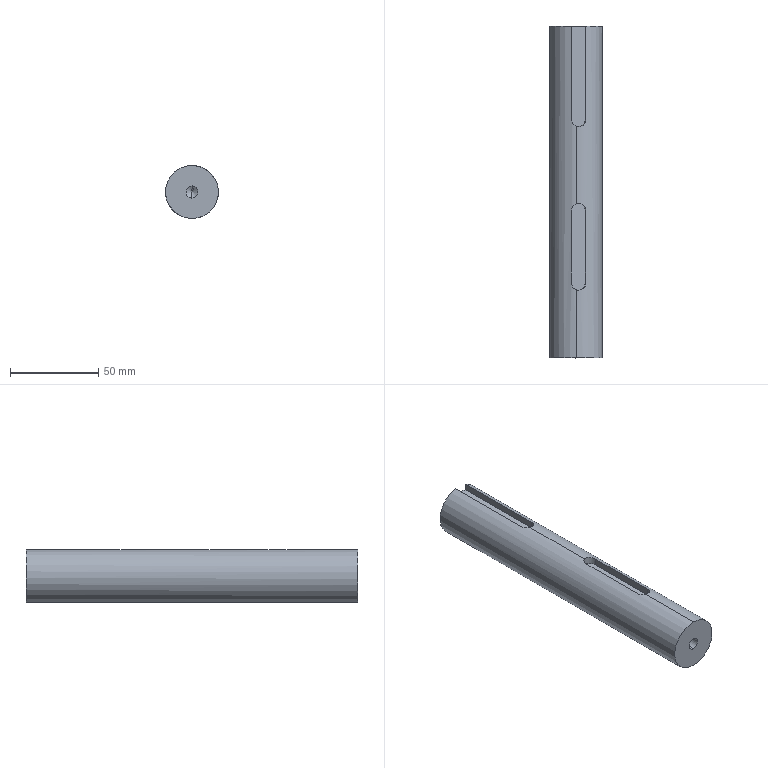Part | SolidWorks | features BaseBody 1 | 1 solid | 21 faces | box 30 x 188 x 30 mm | volume 126976 mm3 | cylinder 9 | plane 8 | cone 4 | commonest cylinder face diameters 6.8 x4 8 x3 30 x2
STEP:
#1=CARTESIAN_POINT('',(-1075.875,-37.235,-89.5));
#2=VERTEX_POINT('',#1);
#3=CARTESIAN_POINT('',(-1075.836,-39.278,-86.1));
#4=VERTEX_POINT('',#3);
#5=CARTESIAN_POINT('',(-1075.836,-39.278,-86.1));
#6=DIRECTION('',(0.009924,-0.515,0.8571));
#7=VECTOR('',#6,1000.);
#8=LINE('',#5,#7);
#9=EDGE_CURVE('',#2,#4,#8,.T.);
#10=ORIENTED_EDGE('',*,*,#9,.F.);
#11=CARTESIAN_POINT('',(-1075.915,-39.278,-92.9));
#12=VERTEX_POINT('',#11);
#13=CARTESIAN_POINT('',(-1075.915,-39.278,-92.9));
#14=DIRECTION('',(-0.009924,-0.515,-0.8571));
#15=VECTOR('',#14,1000.);
#16=LINE('',#13,#15);
#17=EDGE_CURVE('',#2,#12,#16,.T.);
#18=ORIENTED_EDGE('',*,*,#17,.T.);
#19=CARTESIAN_POINT('',(-1075.875,-39.278,-89.5));
#20=DIRECTION('',(0.,-1.,0.));
#21=DIRECTION('',(-0.01158,0.,-0.9999));
#22=AXIS2_PLACEMENT_3D('',#19,#20,#21);
#23=CIRCLE('',#22,3.4);
#24=EDGE_CURVE('',#12,#4,#23,.T.);
#25=ORIENTED_EDGE('',*,*,#24,.T.);
#26=EDGE_LOOP('',(#10,#18,#25));
#27=FACE_OUTER_BOUND('',#26,.T.);
#28=CARTESIAN_POINT('',(-1075.875,-39.278,-89.5));
#29=DIRECTION('',(0.,-1.,0.));
#30=DIRECTION('',(-0.01158,0.,-0.9999));
#31=AXIS2_PLACEMENT_3D('',#28,#29,#30);
#32=CONICAL_SURFACE('',#31,3.4,1.03);
#33=ADVANCED_FACE('',(#27),#32,.F.);
#34=CARTESIAN_POINT('',(-1075.875,77.18,-89.5));
#35=VERTEX_POINT('',#34);
#36=CARTESIAN_POINT('',(-1075.915,79.222,-92.9));
#37=VERTEX_POINT('',#36);
#38=CARTESIAN_POINT('',(-1075.915,79.222,-92.9));
#39=DIRECTION('',(-0.009924,0.515,-0.8571));
#40=VECTOR('',#39,1000.);
#41=LINE('',#38,#40);
#42=EDGE_CURVE('',#35,#37,#41,.T.);
#43=ORIENTED_EDGE('',*,*,#42,.F.);
#44=CARTESIAN_POINT('',(-1075.836,79.222,-86.1));
#45=VERTEX_POINT('',#44);
#46=CARTESIAN_POINT('',(-1075.836,79.222,-86.1));
#47=DIRECTION('',(0.009924,0.515,0.8571));
#48=VECTOR('',#47,1000.);
#49=LINE('',#46,#48);
#50=EDGE_CURVE('',#35,#45,#49,.T.);
#51=ORIENTED_EDGE('',*,*,#50,.T.);
#52=CARTESIAN_POINT('',(-1075.875,79.222,-89.5));
#53=DIRECTION('',(0.,1.,0.));
#54=DIRECTION('',(0.01158,0.,0.9999));
#55=AXIS2_PLACEMENT_3D('',#52,#53,#54);
#56=CIRCLE('',#55,3.4);
#57=EDGE_CURVE('',#45,#37,#56,.T.);
#58=ORIENTED_EDGE('',*,*,#57,.T.);
#59=EDGE_LOOP('',(#43,#51,#58));
#60=FACE_OUTER_BOUND('',#59,.T.);
#61=CARTESIAN_POINT('',(-1075.875,79.222,-89.5));
#62=DIRECTION('',(0.,1.,0.));
#63=DIRECTION('',(0.01158,0.,0.9999));
#64=AXIS2_PLACEMENT_3D('',#61,#62,#63);
#65=CONICAL_SURFACE('',#64,3.4,1.03);
#66=ADVANCED_FACE('',(#60),#65,.F.);
#67=CARTESIAN_POINT('',(-1075.836,-59.028,-86.1));
#68=VERTEX_POINT('',#67);
#69=CARTESIAN_POINT('',(-1075.836,-59.028,-86.1));
#70=DIRECTION('',(0.,-1.,0.));
#71=VECTOR('',#70,1000.);
#72=LINE('',#69,#71);
#73=EDGE_CURVE('',#4,#68,#72,.T.);
#74=ORIENTED_EDGE('',*,*,#73,.F.);
#75=ORIENTED_EDGE('',*,*,#24,.F.);
#76=CARTESIAN_POINT('',(-1075.915,-59.028,-92.9));
#77=VERTEX_POINT('',#76);
#78=CARTESIAN_POINT('',(-1075.915,-59.028,-92.9));
#79=DIRECTION('',(0.,-1.,0.));
#80=VECTOR('',#79,1000.);
#81=LINE('',#78,#80);
#82=EDGE_CURVE('',#12,#77,#81,.T.);
#83=ORIENTED_EDGE('',*,*,#82,.T.);
#84=CARTESIAN_POINT('',(-1075.875,-59.028,-89.5));
#85=DIRECTION('',(0.,-1.,0.));
#86=DIRECTION('',(-0.01158,0.,-0.9999));
#87=AXIS2_PLACEMENT_3D('',#84,#85,#86);
#88=CIRCLE('',#87,3.4);
#89=EDGE_CURVE('',#77,#68,#88,.T.);
#90=ORIENTED_EDGE('',*,*,#89,.T.);
#91=EDGE_LOOP('',(#74,#75,#83,#90));
#92=FACE_OUTER_BOUND('',#91,.T.);
#93=CARTESIAN_POINT('',(-1075.875,-59.028,-89.5));
#94=DIRECTION('',(0.,-1.,0.));
#95=DIRECTION('',(-0.01158,0.,-0.9999));
#96=AXIS2_PLACEMENT_3D('',#93,#94,#95);
#97=CYLINDRICAL_SURFACE('',#96,3.4);
#98=ADVANCED_FACE('',(#92),#97,.F.);
#99=CARTESIAN_POINT('',(-1078.679,-16.675,-78.33));
#100=VERTEX_POINT('',#99);
#101=CARTESIAN_POINT('',(-1070.726,-16.675,-79.198));
#102=VERTEX_POINT('',#101);
#103=CARTESIAN_POINT('',(-1074.703,-16.675,-78.764));
#104=DIRECTION('',(0.1086,0.,0.9941));
#105=DIRECTION('',(-0.9941,0.,0.1086));
#106=AXIS2_PLACEMENT_3D('',#103,#104,#105);
#107=CIRCLE('',#106,4.);
#108=EDGE_CURVE('',#100,#102,#107,.T.);
#109=ORIENTED_EDGE('',*,*,#108,.T.);
#110=CARTESIAN_POINT('',(-1070.726,24.625,-79.198));
#111=VERTEX_POINT('',#110);
#112=CARTESIAN_POINT('',(-1070.726,-16.675,-79.198));
#113=DIRECTION('',(0.,1.,0.));
#114=VECTOR('',#113,1000.);
#115=LINE('',#112,#114);
#116=EDGE_CURVE('',#102,#111,#115,.T.);
#117=ORIENTED_EDGE('',*,*,#116,.T.);
#118=CARTESIAN_POINT('',(-1078.679,24.625,-78.33));
#119=VERTEX_POINT('',#118);
#120=CARTESIAN_POINT('',(-1074.703,24.625,-78.764));
#121=DIRECTION('',(0.1086,0.,0.9941));
#122=DIRECTION('',(-0.9941,0.,0.1086));
#123=AXIS2_PLACEMENT_3D('',#120,#121,#122);
#124=CIRCLE('',#123,4.);
#125=EDGE_CURVE('',#111,#119,#124,.T.);
#126=ORIENTED_EDGE('',*,*,#125,.T.);
#127=CARTESIAN_POINT('',(-1078.679,24.625,-78.33));
#128=DIRECTION('',(0.,-1.,0.));
#129=VECTOR('',#128,1000.);
#130=LINE('',#127,#129);
#131=EDGE_CURVE('',#119,#100,#130,.T.);
#132=ORIENTED_EDGE('',*,*,#131,.T.);
#133=EDGE_LOOP('',(#109,#117,#126,#132));
#134=FACE_OUTER_BOUND('',#133,.T.);
#135=CARTESIAN_POINT('',(-1074.703,24.625,-78.764));
#136=DIRECTION('',(0.1086,0.,0.9941));
#137=DIRECTION('',(0.,1.,0.));
#138=AXIS2_PLACEMENT_3D('',#135,#136,#137);
#139=PLANE('',#138);
#140=ADVANCED_FACE('',(#134),#139,.T.);
#141=CARTESIAN_POINT('',(-1070.329,24.625,-75.563));
#142=VERTEX_POINT('',#141);
#143=CARTESIAN_POINT('',(-1070.726,24.625,-79.198));
#144=DIRECTION('',(-0.1086,0.,-0.9941));
#145=VECTOR('',#144,1000.);
#146=LINE('',#143,#145);
#147=EDGE_CURVE('',#142,#111,#146,.T.);
#148=ORIENTED_EDGE('',*,*,#147,.T.);
#149=ORIENTED_EDGE('',*,*,#116,.F.);
#150=CARTESIAN_POINT('',(-1070.329,-16.675,-75.563));
#151=VERTEX_POINT('',#150);
#152=CARTESIAN_POINT('',(-1070.726,-16.675,-79.198));
#153=DIRECTION('',(0.1086,0.,0.9941));
#154=VECTOR('',#153,1000.);
#155=LINE('',#152,#154);
#156=EDGE_CURVE('',#102,#151,#155,.T.);
#157=ORIENTED_EDGE('',*,*,#156,.T.);
#158=CARTESIAN_POINT('',(-1070.329,-91.028,-75.563));
#159=DIRECTION('',(0.,-1.,0.));
#160=VECTOR('',#159,1000.);
#161=LINE('',#158,#160);
#162=EDGE_CURVE('',#142,#151,#161,.T.);
#163=ORIENTED_EDGE('',*,*,#162,.F.);
#164=EDGE_LOOP('',(#148,#149,#157,#163));
#165=FACE_OUTER_BOUND('',#164,.T.);
#166=CARTESIAN_POINT('',(-1070.726,-16.675,-79.198));
#167=DIRECTION('',(0.9941,0.,-0.1086));
#168=DIRECTION('',(0.,1.,0.));
#169=AXIS2_PLACEMENT_3D('',#166,#167,#168);
#170=PLANE('',#169);
#171=ADVANCED_FACE('',(#165),#170,.F.);
#172=CARTESIAN_POINT('',(-1075.915,128.972,-92.9));
#173=VERTEX_POINT('',#172);
#174=CARTESIAN_POINT('',(-1075.915,98.972,-92.9));
#175=DIRECTION('',(0.,1.,0.));
#176=VECTOR('',#175,1000.);
#177=LINE('',#174,#176);
#178=EDGE_CURVE('',#37,#173,#177,.T.);
#179=ORIENTED_EDGE('',*,*,#178,.F.);
#180=ORIENTED_EDGE('',*,*,#57,.F.);
#181=CARTESIAN_POINT('',(-1075.836,128.972,-86.1));
#182=VERTEX_POINT('',#181);
#183=CARTESIAN_POINT('',(-1075.836,98.972,-86.1));
#184=DIRECTION('',(0.,1.,0.));
#185=VECTOR('',#184,1000.);
#186=LINE('',#183,#185);
#187=EDGE_CURVE('',#45,#182,#186,.T.);
#188=ORIENTED_EDGE('',*,*,#187,.T.);
#189=CARTESIAN_POINT('',(-1075.875,128.972,-89.5));
#190=DIRECTION('',(0.,-1.,0.));
#191=DIRECTION('',(0.01158,0.,0.9999));
#192=AXIS2_PLACEMENT_3D('',#189,#190,#191);
#193=CIRCLE('',#192,3.4);
#194=EDGE_CURVE('',#173,#182,#193,.T.);
#195=ORIENTED_EDGE('',*,*,#194,.F.);
#196=EDGE_LOOP('',(#179,#180,#188,#195));
#197=FACE_OUTER_BOUND('',#196,.T.);
#198=CARTESIAN_POINT('',(-1075.875,98.972,-89.5));
#199=DIRECTION('',(0.,1.,0.));
#200=DIRECTION('',(0.01158,0.,0.9999));
#201=AXIS2_PLACEMENT_3D('',#198,#199,#200);
#202=CYLINDRICAL_SURFACE('',#201,3.4);
#203=ADVANCED_FACE('',(#197),#202,.F.);
#204=CARTESIAN_POINT('',(-1070.726,128.972,-79.198));
#205=VERTEX_POINT('',#204);
#206=CARTESIAN_POINT('',(-1070.329,128.972,-75.563));
#207=VERTEX_POINT('',#206);
#208=CARTESIAN_POINT('',(-1070.726,128.972,-79.198));
#209=DIRECTION('',(0.1086,0.,0.9941));
#210=VECTOR('',#209,1000.);
#211=LINE('',#208,#210);
#212=EDGE_CURVE('',#205,#207,#211,.T.);
#213=ORIENTED_EDGE('',*,*,#212,.F.);
#214=CARTESIAN_POINT('',(-1070.726,75.972,-79.198));
#215=VERTEX_POINT('',#214);
#216=CARTESIAN_POINT('',(-1070.726,75.972,-79.198));
#217=DIRECTION('',(0.,1.,0.));
#218=VECTOR('',#217,1000.);
#219=LINE('',#216,#218);
#220=EDGE_CURVE('',#215,#205,#219,.T.);
#221=ORIENTED_EDGE('',*,*,#220,.F.);
#222=CARTESIAN_POINT('',(-1070.329,75.972,-75.563));
#223=VERTEX_POINT('',#222);
#224=CARTESIAN_POINT('',(-1070.726,75.972,-79.198));
#225=DIRECTION('',(0.1086,0.,0.9941));
#226=VECTOR('',#225,1000.);
#227=LINE('',#224,#226);
#228=EDGE_CURVE('',#215,#223,#227,.T.);
#229=ORIENTED_EDGE('',*,*,#228,.T.);
#230=CARTESIAN_POINT('',(-1070.329,-91.028,-75.563));
#231=DIRECTION('',(0.,-1.,0.));
#232=VECTOR('',#231,1000.);
#233=LINE('',#230,#232);
#234=EDGE_CURVE('',#207,#223,#233,.T.);
#235=ORIENTED_EDGE('',*,*,#234,.F.);
#236=EDGE_LOOP('',(#213,#221,#229,#235));
#237=FACE_OUTER_BOUND('',#236,.T.);
#238=CARTESIAN_POINT('',(-1070.726,75.972,-79.198));
#239=DIRECTION('',(0.9941,0.,-0.1086));
#240=DIRECTION('',(0.,1.,0.));
#241=AXIS2_PLACEMENT_3D('',#238,#239,#240);
#242=PLANE('',#241);
#243=ADVANCED_FACE('',(#237),#242,.F.);
#244=CARTESIAN_POINT('',(-1078.679,75.972,-78.33));
#245=VERTEX_POINT('',#244);
#246=CARTESIAN_POINT('',(-1074.703,75.972,-78.764));
#247=DIRECTION('',(0.1086,0.,0.9941));
#248=DIRECTION('',(-0.9941,0.,0.1086));
#249=AXIS2_PLACEMENT_3D('',#246,#247,#248);
#250=CIRCLE('',#249,4.);
#251=EDGE_CURVE('',#245,#215,#250,.T.);
#252=ORIENTED_EDGE('',*,*,#251,.T.);
#253=ORIENTED_EDGE('',*,*,#220,.T.);
#254=CARTESIAN_POINT('',(-1078.679,128.972,-78.33));
#255=VERTEX_POINT('',#254);
#256=CARTESIAN_POINT('',(-1074.703,128.972,-78.764));
#257=DIRECTION('',(0.9941,0.,-0.1086));
#258=VECTOR('',#257,1000.);
#259=LINE('',#256,#258);
#260=EDGE_CURVE('',#255,#205,#259,.T.);
#261=ORIENTED_EDGE('',*,*,#260,.F.);
#262=CARTESIAN_POINT('',(-1078.679,98.972,-78.33));
#263=DIRECTION('',(0.,-1.,0.));
#264=VECTOR('',#263,1000.);
#265=LINE('',#262,#264);
#266=EDGE_CURVE('',#255,#245,#265,.T.);
#267=ORIENTED_EDGE('',*,*,#266,.T.);
#268=EDGE_LOOP('',(#252,#253,#261,#267));
#269=FACE_OUTER_BOUND('',#268,.T.);
#270=CARTESIAN_POINT('',(-1074.703,75.972,-78.764));
#271=DIRECTION('',(0.1086,0.,0.9941));
#272=DIRECTION('',(0.,1.,0.));
#273=AXIS2_PLACEMENT_3D('',#270,#271,#272);
#274=PLANE('',#273);
#275=ADVANCED_FACE('',(#269),#274,.T.);
#276=CARTESIAN_POINT('',(-1075.702,-59.028,-74.501));
#277=VERTEX_POINT('',#276);
#278=CARTESIAN_POINT('',(-1076.049,-59.028,-104.499));
#279=VERTEX_POINT('',#278);
#280=CARTESIAN_POINT('',(-1075.875,-59.028,-89.5));
#281=DIRECTION('',(0.,1.,0.));
#282=DIRECTION('',(0.01158,0.,0.9999));
#283=AXIS2_PLACEMENT_3D('',#280,#281,#282);
#284=CIRCLE('',#283,15.);
#285=EDGE_CURVE('',#277,#279,#284,.T.);
#286=ORIENTED_EDGE('',*,*,#285,.F.);
#287=CARTESIAN_POINT('',(-1075.875,-59.028,-89.5));
#288=DIRECTION('',(0.,1.,0.));
#289=DIRECTION('',(0.01158,0.,0.9999));
#290=AXIS2_PLACEMENT_3D('',#287,#288,#289);
#291=CIRCLE('',#290,15.);
#292=EDGE_CURVE('',#279,#277,#291,.T.);
#293=ORIENTED_EDGE('',*,*,#292,.F.);
#294=EDGE_LOOP('',(#286,#293));
#295=FACE_OUTER_BOUND('',#294,.T.);
#296=ORIENTED_EDGE('',*,*,#89,.F.);
#297=CARTESIAN_POINT('',(-1075.875,-59.028,-89.5));
#298=DIRECTION('',(0.,-1.,0.));
#299=DIRECTION('',(-0.01158,0.,-0.9999));
#300=AXIS2_PLACEMENT_3D('',#297,#298,#299);
#301=CIRCLE('',#300,3.4);
#302=EDGE_CURVE('',#68,#77,#301,.T.);
#303=ORIENTED_EDGE('',*,*,#302,.F.);
#304=EDGE_LOOP('',(#296,#303));
#305=FACE_BOUND('',#304,.T.);
#306=CARTESIAN_POINT('',(-1075.875,-59.028,-89.5));
#307=DIRECTION('',(0.,1.,0.));
#308=DIRECTION('',(0.01158,0.,0.9999));
#309=AXIS2_PLACEMENT_3D('',#306,#307,#308);
#310=PLANE('',#309);
#311=ADVANCED_FACE('',(#295,#305),#310,.F.);
#312=ORIENTED_EDGE('',*,*,#156,.F.);
#313=ORIENTED_EDGE('',*,*,#108,.F.);
#314=CARTESIAN_POINT('',(-1078.282,-16.675,-74.694));
#315=VERTEX_POINT('',#314);
#316=CARTESIAN_POINT('',(-1078.679,-16.675,-78.33));
#317=DIRECTION('',(0.1086,0.,0.9941));
#318=VECTOR('',#317,1000.);
#319=LINE('',#316,#318);
#320=EDGE_CURVE('',#100,#315,#319,.T.);
#321=ORIENTED_EDGE('',*,*,#320,.T.);
#322=CARTESIAN_POINT('',(-1075.702,-20.401,-74.501));
#323=VERTEX_POINT('',#322);
#324=CARTESIAN_POINT('',(-1075.702,-20.401,-74.501));
#325=CARTESIAN_POINT('',(-1076.077,-20.255,-74.497));
#326=CARTESIAN_POINT('',(-1076.424,-20.057,-74.507));
#327=CARTESIAN_POINT('',(-1076.901,-19.683,-74.534));
#328=CARTESIAN_POINT('',(-1077.049,-19.548,-74.545));
#329=CARTESIAN_POINT('',(-1077.324,-19.258,-74.569));
#330=CARTESIAN_POINT('',(-1077.449,-19.104,-74.582));
#331=CARTESIAN_POINT('',(-1077.681,-18.772,-74.609));
#332=CARTESIAN_POINT('',(-1077.784,-18.599,-74.622));
#333=CARTESIAN_POINT('',(-1077.917,-18.331,-74.639));
#334=CARTESIAN_POINT('',(-1077.957,-18.24,-74.645));
#335=CARTESIAN_POINT('',(-1078.032,-18.055,-74.656));
#336=CARTESIAN_POINT('',(-1078.066,-17.962,-74.661));
#337=CARTESIAN_POINT('',(-1078.22,-17.477,-74.684));
#338=CARTESIAN_POINT('',(-1078.282,-17.08,-74.694));
#339=CARTESIAN_POINT('',(-1078.282,-16.675,-74.694));
#340=B_SPLINE_CURVE_WITH_KNOTS('',3,(#324,#325,#326,#327,#328,#329,#330,#331,#332,#333,#334,#335,#336,#337,#338,#339),.UNSPECIFIED.,.F.,.F.,(4,2,2,2,2,2,2,4),(0.,0.25,0.375,0.5,0.625,0.6875,0.75,1.),.UNSPECIFIED.);
#341=EDGE_CURVE('',#323,#315,#340,.T.);
#342=ORIENTED_EDGE('',*,*,#341,.F.);
#343=CARTESIAN_POINT('',(-1070.329,-16.675,-75.563));
#344=CARTESIAN_POINT('',(-1070.329,-17.001,-75.563));
#345=CARTESIAN_POINT('',(-1070.367,-17.323,-75.548));
#346=CARTESIAN_POINT('',(-1070.481,-17.797,-75.504));
#347=CARTESIAN_POINT('',(-1070.527,-17.951,-75.486));
#348=CARTESIAN_POINT('',(-1070.639,-18.253,-75.444));
#349=CARTESIAN_POINT('',(-1070.704,-18.402,-75.419));
#350=CARTESIAN_POINT('',(-1070.851,-18.688,-75.366));
#351=CARTESIAN_POINT('',(-1070.932,-18.826,-75.338));
#352=CARTESIAN_POINT('',(-1071.11,-19.09,-75.277));
#353=CARTESIAN_POINT('',(-1071.208,-19.218,-75.244));
#354=CARTESIAN_POINT('',(-1071.521,-19.579,-75.144));
#355=CARTESIAN_POINT('',(-1071.755,-19.791,-75.074));
#356=CARTESIAN_POINT('',(-1072.279,-20.158,-74.935));
#357=CARTESIAN_POINT('',(-1072.557,-20.306,-74.868));
#358=CARTESIAN_POINT('',(-1073.158,-20.535,-74.745));
#359=CARTESIAN_POINT('',(-1073.469,-20.611,-74.691));
#360=CARTESIAN_POINT('',(-1074.112,-20.686,-74.6));
#361=CARTESIAN_POINT('',(-1074.434,-20.684,-74.566));
#362=CARTESIAN_POINT('',(-1075.081,-20.6,-74.518));
#363=CARTESIAN_POINT('',(-1075.396,-20.52,-74.505));
#364=CARTESIAN_POINT('',(-1075.702,-20.401,-74.501));
#365=B_SPLINE_CURVE_WITH_KNOTS('',3,(#343,#344,#345,#346,#347,#348,#349,#350,#351,#352,#353,#354,#355,#356,#357,#358,#359,#360,#361,#362,#363,#364),.UNSPECIFIED.,.F.,.F.,(4,2,2,2,2,2,2,2,2,2,4),(0.,0.125,0.1875,0.25,0.3125,0.375,0.5,0.625,0.75,0.875,1.),.UNSPECIFIED.);
#366=EDGE_CURVE('',#151,#323,#365,.T.);
#367=ORIENTED_EDGE('',*,*,#366,.F.);
#368=EDGE_LOOP('',(#312,#313,#321,#342,#367));
#369=FACE_OUTER_BOUND('',#368,.T.);
#370=CARTESIAN_POINT('',(-1074.703,-16.675,-78.764));
#371=DIRECTION('',(0.1086,0.,0.9941));
#372=DIRECTION('',(-0.9941,0.,0.1086));
#373=AXIS2_PLACEMENT_3D('',#370,#371,#372);
#374=CYLINDRICAL_SURFACE('',#373,4.);
#375=ADVANCED_FACE('',(#369),#374,.F.);
#376=ORIENTED_EDGE('',*,*,#320,.F.);
#377=ORIENTED_EDGE('',*,*,#131,.F.);
#378=CARTESIAN_POINT('',(-1078.282,24.625,-74.694));
#379=VERTEX_POINT('',#378);
#380=CARTESIAN_POINT('',(-1078.679,24.625,-78.33));
#381=DIRECTION('',(0.1086,0.,0.9941));
#382=VECTOR('',#381,1000.);
#383=LINE('',#380,#382);
#384=EDGE_CURVE('',#119,#379,#383,.T.);
#385=ORIENTED_EDGE('',*,*,#384,.T.);
#386=CARTESIAN_POINT('',(-1078.282,-91.028,-74.694));
#387=DIRECTION('',(0.,1.,0.));
#388=VECTOR('',#387,1000.);
#389=LINE('',#386,#388);
#390=EDGE_CURVE('',#315,#379,#389,.T.);
#391=ORIENTED_EDGE('',*,*,#390,.F.);
#392=EDGE_LOOP('',(#376,#377,#385,#391));
#393=FACE_OUTER_BOUND('',#392,.T.);
#394=CARTESIAN_POINT('',(-1078.679,24.625,-78.33));
#395=DIRECTION('',(-0.9941,0.,0.1086));
#396=DIRECTION('',(-0.1086,0.,-0.9941));
#397=AXIS2_PLACEMENT_3D('',#394,#395,#396);
#398=PLANE('',#397);
#399=ADVANCED_FACE('',(#393),#398,.F.);
#400=ORIENTED_EDGE('',*,*,#384,.F.);
#401=ORIENTED_EDGE('',*,*,#125,.F.);
#402=ORIENTED_EDGE('',*,*,#147,.F.);
#403=CARTESIAN_POINT('',(-1075.702,28.351,-74.501));
#404=VERTEX_POINT('',#403);
#405=CARTESIAN_POINT('',(-1075.702,28.351,-74.501));
#406=CARTESIAN_POINT('',(-1075.397,28.469,-74.505));
#407=CARTESIAN_POINT('',(-1075.085,28.549,-74.517));
#408=CARTESIAN_POINT('',(-1074.438,28.634,-74.566));
#409=CARTESIAN_POINT('',(-1074.114,28.636,-74.6));
#410=CARTESIAN_POINT('',(-1073.632,28.58,-74.668));
#411=CARTESIAN_POINT('',(-1073.474,28.552,-74.693));
#412=CARTESIAN_POINT('',(-1073.163,28.476,-74.746));
#413=CARTESIAN_POINT('',(-1073.009,28.428,-74.776));
#414=CARTESIAN_POINT('',(-1072.561,28.257,-74.868));
#415=CARTESIAN_POINT('',(-1072.28,28.109,-74.935));
#416=CARTESIAN_POINT('',(-1071.758,27.743,-75.074));
#417=CARTESIAN_POINT('',(-1071.524,27.532,-75.143));
#418=CARTESIAN_POINT('',(-1071.208,27.168,-75.244));
#419=CARTESIAN_POINT('',(-1071.111,27.041,-75.276));
#420=CARTESIAN_POINT('',(-1070.933,26.777,-75.337));
#421=CARTESIAN_POINT('',(-1070.852,26.64,-75.366));
#422=CARTESIAN_POINT('',(-1070.704,26.352,-75.419));
#423=CARTESIAN_POINT('',(-1070.639,26.204,-75.443));
#424=CARTESIAN_POINT('',(-1070.528,25.903,-75.485));
#425=CARTESIAN_POINT('',(-1070.482,25.75,-75.503));
#426=CARTESIAN_POINT('',(-1070.367,25.274,-75.548));
#427=CARTESIAN_POINT('',(-1070.329,24.951,-75.563));
#428=CARTESIAN_POINT('',(-1070.329,24.625,-75.563));
#429=B_SPLINE_CURVE_WITH_KNOTS('',3,(#405,#406,#407,#408,#409,#410,#411,#412,#413,#414,#415,#416,#417,#418,#419,#420,#421,#422,#423,#424,#425,#426,#427,#428),.UNSPECIFIED.,.F.,.F.,(4,2,2,2,2,2,2,2,2,2,2,4),(0.,0.125,0.25,0.3125,0.375,0.5,0.625,0.6875,0.75,0.8125,0.875,1.),.UNSPECIFIED.);
#430=EDGE_CURVE('',#404,#142,#429,.T.);
#431=ORIENTED_EDGE('',*,*,#430,.F.);
#432=CARTESIAN_POINT('',(-1078.282,24.625,-74.694));
#433=CARTESIAN_POINT('',(-1078.282,24.826,-74.694));
#434=CARTESIAN_POINT('',(-1078.267,25.026,-74.692));
#435=CARTESIAN_POINT('',(-1078.206,25.42,-74.682));
#436=CARTESIAN_POINT('',(-1078.159,25.617,-74.675));
#437=CARTESIAN_POINT('',(-1078.038,26.,-74.657));
#438=CARTESIAN_POINT('',(-1077.964,26.185,-74.646));
#439=CARTESIAN_POINT('',(-1077.787,26.543,-74.622));
#440=CARTESIAN_POINT('',(-1077.684,26.717,-74.609));
#441=CARTESIAN_POINT('',(-1077.339,27.212,-74.57));
#442=CARTESIAN_POINT('',(-1077.067,27.501,-74.544));
#443=CARTESIAN_POINT('',(-1076.428,28.004,-74.507));
#444=CARTESIAN_POINT('',(-1076.079,28.204,-74.497));
#445=CARTESIAN_POINT('',(-1075.702,28.351,-74.501));
#446=B_SPLINE_CURVE_WITH_KNOTS('',3,(#432,#433,#434,#435,#436,#437,#438,#439,#440,#441,#442,#443,#444,#445),.UNSPECIFIED.,.F.,.F.,(4,2,2,2,2,2,4),(0.,0.125,0.25,0.375,0.5,0.75,1.),.UNSPECIFIED.);
#447=EDGE_CURVE('',#379,#404,#446,.T.);
#448=ORIENTED_EDGE('',*,*,#447,.F.);
#449=EDGE_LOOP('',(#400,#401,#402,#431,#448));
#450=FACE_OUTER_BOUND('',#449,.T.);
#451=CARTESIAN_POINT('',(-1074.703,24.625,-78.764));
#452=DIRECTION('',(0.1086,0.,0.9941));
#453=DIRECTION('',(-0.9941,0.,0.1086));
#454=AXIS2_PLACEMENT_3D('',#451,#452,#453);
#455=CYLINDRICAL_SURFACE('',#454,4.);
#456=ADVANCED_FACE('',(#450),#455,.F.);
#457=ORIENTED_EDGE('',*,*,#228,.F.);
#458=ORIENTED_EDGE('',*,*,#251,.F.);
#459=CARTESIAN_POINT('',(-1078.282,75.972,-74.694));
#460=VERTEX_POINT('',#459);
#461=CARTESIAN_POINT('',(-1078.679,75.972,-78.33));
#462=DIRECTION('',(0.1086,0.,0.9941));
#463=VECTOR('',#462,1000.);
#464=LINE('',#461,#463);
#465=EDGE_CURVE('',#245,#460,#464,.T.);
#466=ORIENTED_EDGE('',*,*,#465,.T.);
#467=CARTESIAN_POINT('',(-1075.702,72.247,-74.501));
#468=VERTEX_POINT('',#467);
#469=CARTESIAN_POINT('',(-1075.702,72.247,-74.501));
#470=CARTESIAN_POINT('',(-1076.077,72.393,-74.497));
#471=CARTESIAN_POINT('',(-1076.424,72.59,-74.507));
#472=CARTESIAN_POINT('',(-1076.901,72.965,-74.534));
#473=CARTESIAN_POINT('',(-1077.049,73.1,-74.545));
#474=CARTESIAN_POINT('',(-1077.324,73.39,-74.569));
#475=CARTESIAN_POINT('',(-1077.449,73.543,-74.582));
#476=CARTESIAN_POINT('',(-1077.681,73.876,-74.609));
#477=CARTESIAN_POINT('',(-1077.784,74.048,-74.622));
#478=CARTESIAN_POINT('',(-1077.917,74.317,-74.639));
#479=CARTESIAN_POINT('',(-1077.957,74.408,-74.645));
#480=CARTESIAN_POINT('',(-1078.032,74.593,-74.656));
#481=CARTESIAN_POINT('',(-1078.066,74.685,-74.661));
#482=CARTESIAN_POINT('',(-1078.22,75.171,-74.684));
#483=CARTESIAN_POINT('',(-1078.282,75.567,-74.694));
#484=CARTESIAN_POINT('',(-1078.282,75.972,-74.694));
#485=B_SPLINE_CURVE_WITH_KNOTS('',3,(#469,#470,#471,#472,#473,#474,#475,#476,#477,#478,#479,#480,#481,#482,#483,#484),.UNSPECIFIED.,.F.,.F.,(4,2,2,2,2,2,2,4),(0.,0.25,0.375,0.5,0.625,0.6875,0.75,1.),.UNSPECIFIED.);
#486=EDGE_CURVE('',#468,#460,#485,.T.);
#487=ORIENTED_EDGE('',*,*,#486,.F.);
#488=CARTESIAN_POINT('',(-1070.329,75.972,-75.563));
#489=CARTESIAN_POINT('',(-1070.329,75.647,-75.563));
#490=CARTESIAN_POINT('',(-1070.367,75.324,-75.548));
#491=CARTESIAN_POINT('',(-1070.481,74.851,-75.504));
#492=CARTESIAN_POINT('',(-1070.527,74.697,-75.486));
#493=CARTESIAN_POINT('',(-1070.639,74.395,-75.444));
#494=CARTESIAN_POINT('',(-1070.704,74.245,-75.419));
#495=CARTESIAN_POINT('',(-1070.851,73.959,-75.366));
#496=CARTESIAN_POINT('',(-1070.932,73.822,-75.338));
#497=CARTESIAN_POINT('',(-1071.11,73.557,-75.277));
#498=CARTESIAN_POINT('',(-1071.208,73.429,-75.244));
#499=CARTESIAN_POINT('',(-1071.521,73.068,-75.144));
#500=CARTESIAN_POINT('',(-1071.755,72.857,-75.074));
#501=CARTESIAN_POINT('',(-1072.279,72.49,-74.935));
#502=CARTESIAN_POINT('',(-1072.557,72.342,-74.868));
#503=CARTESIAN_POINT('',(-1073.158,72.112,-74.745));
#504=CARTESIAN_POINT('',(-1073.469,72.036,-74.691));
#505=CARTESIAN_POINT('',(-1074.112,71.961,-74.6));
#506=CARTESIAN_POINT('',(-1074.434,71.964,-74.566));
#507=CARTESIAN_POINT('',(-1075.081,72.047,-74.518));
#508=CARTESIAN_POINT('',(-1075.396,72.128,-74.505));
#509=CARTESIAN_POINT('',(-1075.702,72.247,-74.501));
#510=B_SPLINE_CURVE_WITH_KNOTS('',3,(#488,#489,#490,#491,#492,#493,#494,#495,#496,#497,#498,#499,#500,#501,#502,#503,#504,#505,#506,#507,#508,#509),.UNSPECIFIED.,.F.,.F.,(4,2,2,2,2,2,2,2,2,2,4),(0.,0.125,0.1875,0.25,0.3125,0.375,0.5,0.625,0.75,0.875,1.),.UNSPECIFIED.);
#511=EDGE_CURVE('',#223,#468,#510,.T.);
#512=ORIENTED_EDGE('',*,*,#511,.F.);
#513=EDGE_LOOP('',(#457,#458,#466,#487,#512));
#514=FACE_OUTER_BOUND('',#513,.T.);
#515=CARTESIAN_POINT('',(-1074.703,75.972,-78.764));
#516=DIRECTION('',(0.1086,0.,0.9941));
#517=DIRECTION('',(-0.9941,0.,0.1086));
#518=AXIS2_PLACEMENT_3D('',#515,#516,#517);
#519=CYLINDRICAL_SURFACE('',#518,4.);
#520=ADVANCED_FACE('',(#514),#519,.F.);
#521=ORIENTED_EDGE('',*,*,#465,.F.);
#522=ORIENTED_EDGE('',*,*,#266,.F.);
#523=CARTESIAN_POINT('',(-1078.282,128.972,-74.694));
#524=VERTEX_POINT('',#523);
#525=CARTESIAN_POINT('',(-1078.679,128.972,-78.33));
#526=DIRECTION('',(-0.1086,0.,-0.9941));
#527=VECTOR('',#526,1000.);
#528=LINE('',#525,#527);
#529=EDGE_CURVE('',#524,#255,#528,.T.);
#530=ORIENTED_EDGE('',*,*,#529,.F.);
#531=CARTESIAN_POINT('',(-1078.282,-91.028,-74.694));
#532=DIRECTION('',(0.,1.,0.));
#533=VECTOR('',#532,1000.);
#534=LINE('',#531,#533);
#535=EDGE_CURVE('',#460,#524,#534,.T.);
#536=ORIENTED_EDGE('',*,*,#535,.F.);
#537=EDGE_LOOP('',(#521,#522,#530,#536));
#538=FACE_OUTER_BOUND('',#537,.T.);
#539=CARTESIAN_POINT('',(-1078.679,98.972,-78.33));
#540=DIRECTION('',(-0.9941,0.,0.1086));
#541=DIRECTION('',(-0.1086,0.,-0.9941));
#542=AXIS2_PLACEMENT_3D('',#539,#540,#541);
#543=PLANE('',#542);
#544=ADVANCED_FACE('',(#538),#543,.F.);
#545=ORIENTED_EDGE('',*,*,#529,.T.);
#546=ORIENTED_EDGE('',*,*,#260,.T.);
#547=ORIENTED_EDGE('',*,*,#212,.T.);
#548=CARTESIAN_POINT('',(-1076.049,128.972,-104.499));
#549=VERTEX_POINT('',#548);
#550=CARTESIAN_POINT('',(-1075.875,128.972,-89.5));
#551=DIRECTION('',(0.,-1.,0.));
#552=DIRECTION('',(0.01158,0.,0.9999));
#553=AXIS2_PLACEMENT_3D('',#550,#551,#552);
#554=CIRCLE('',#553,15.);
#555=EDGE_CURVE('',#549,#207,#554,.T.);
#556=ORIENTED_EDGE('',*,*,#555,.F.);
#557=CARTESIAN_POINT('',(-1075.875,128.972,-89.5));
#558=DIRECTION('',(0.,-1.,0.));
#559=DIRECTION('',(0.01158,0.,0.9999));
#560=AXIS2_PLACEMENT_3D('',#557,#558,#559);
#561=CIRCLE('',#560,15.);
#562=EDGE_CURVE('',#524,#549,#561,.T.);
#563=ORIENTED_EDGE('',*,*,#562,.F.);
#564=EDGE_LOOP('',(#545,#546,#547,#556,#563));
#565=FACE_OUTER_BOUND('',#564,.T.);
#566=CARTESIAN_POINT('',(-1075.875,128.972,-89.5));
#567=DIRECTION('',(0.,-1.,0.));
#568=DIRECTION('',(0.01158,0.,0.9999));
#569=AXIS2_PLACEMENT_3D('',#566,#567,#568);
#570=CIRCLE('',#569,3.4);
#571=EDGE_CURVE('',#182,#173,#570,.T.);
#572=ORIENTED_EDGE('',*,*,#571,.T.);
#573=ORIENTED_EDGE('',*,*,#194,.T.);
#574=EDGE_LOOP('',(#572,#573));
#575=FACE_BOUND('',#574,.T.);
#576=CARTESIAN_POINT('',(-1075.875,128.972,-89.5));
#577=DIRECTION('',(0.,1.,0.));
#578=DIRECTION('',(0.01158,0.,0.9999));
#579=AXIS2_PLACEMENT_3D('',#576,#577,#578);
#580=PLANE('',#579);
#581=ADVANCED_FACE('',(#565,#575),#580,.T.);
#582=CARTESIAN_POINT('',(-1076.049,-91.028,-104.499));
#583=DIRECTION('',(0.,1.,0.));
#584=VECTOR('',#583,1000.);
#585=LINE('',#582,#584);
#586=EDGE_CURVE('',#279,#549,#585,.T.);
#587=ORIENTED_EDGE('',*,*,#586,.F.);
#588=ORIENTED_EDGE('',*,*,#292,.T.);
#589=CARTESIAN_POINT('',(-1075.702,-91.028,-74.501));
#590=DIRECTION('',(0.,1.,0.));
#591=VECTOR('',#590,1000.);
#592=LINE('',#589,#591);
#593=EDGE_CURVE('',#277,#323,#592,.T.);
#594=ORIENTED_EDGE('',*,*,#593,.T.);
#595=ORIENTED_EDGE('',*,*,#341,.T.);
#596=ORIENTED_EDGE('',*,*,#390,.T.);
#597=ORIENTED_EDGE('',*,*,#447,.T.);
#598=CARTESIAN_POINT('',(-1075.702,-91.028,-74.501));
#599=DIRECTION('',(0.,1.,0.));
#600=VECTOR('',#599,1000.);
#601=LINE('',#598,#600);
#602=EDGE_CURVE('',#404,#468,#601,.T.);
#603=ORIENTED_EDGE('',*,*,#602,.T.);
#604=ORIENTED_EDGE('',*,*,#486,.T.);
#605=ORIENTED_EDGE('',*,*,#535,.T.);
#606=ORIENTED_EDGE('',*,*,#562,.T.);
#607=EDGE_LOOP('',(#587,#588,#594,#595,#596,#597,#603,#604,#605,#606));
#608=FACE_OUTER_BOUND('',#607,.T.);
#609=CARTESIAN_POINT('',(-1075.875,-91.028,-89.5));
#610=DIRECTION('',(0.,1.,0.));
#611=DIRECTION('',(0.01158,0.,0.9999));
#612=AXIS2_PLACEMENT_3D('',#609,#610,#611);
#613=CYLINDRICAL_SURFACE('',#612,15.);
#614=ADVANCED_FACE('',(#608),#613,.T.);
#615=ORIENTED_EDGE('',*,*,#17,.F.);
#616=ORIENTED_EDGE('',*,*,#9,.T.);
#617=CARTESIAN_POINT('',(-1075.875,-39.278,-89.5));
#618=DIRECTION('',(0.,-1.,0.));
#619=DIRECTION('',(-0.01158,0.,-0.9999));
#620=AXIS2_PLACEMENT_3D('',#617,#618,#619);
#621=CIRCLE('',#620,3.4);
#622=EDGE_CURVE('',#4,#12,#621,.T.);
#623=ORIENTED_EDGE('',*,*,#622,.T.);
#624=EDGE_LOOP('',(#615,#616,#623));
#625=FACE_OUTER_BOUND('',#624,.T.);
#626=CARTESIAN_POINT('',(-1075.875,-39.278,-89.5));
#627=DIRECTION('',(0.,-1.,0.));
#628=DIRECTION('',(-0.01158,0.,-0.9999));
#629=AXIS2_PLACEMENT_3D('',#626,#627,#628);
#630=CONICAL_SURFACE('',#629,3.4,1.03);
#631=ADVANCED_FACE('',(#625),#630,.F.);
#632=ORIENTED_EDGE('',*,*,#50,.F.);
#633=ORIENTED_EDGE('',*,*,#42,.T.);
#634=CARTESIAN_POINT('',(-1075.875,79.222,-89.5));
#635=DIRECTION('',(0.,1.,0.));
#636=DIRECTION('',(0.01158,0.,0.9999));
#637=AXIS2_PLACEMENT_3D('',#634,#635,#636);
#638=CIRCLE('',#637,3.4);
#639=EDGE_CURVE('',#37,#45,#638,.T.);
#640=ORIENTED_EDGE('',*,*,#639,.T.);
#641=EDGE_LOOP('',(#632,#633,#640));
#642=FACE_OUTER_BOUND('',#641,.T.);
#643=CARTESIAN_POINT('',(-1075.875,79.222,-89.5));
#644=DIRECTION('',(0.,1.,0.));
#645=DIRECTION('',(0.01158,0.,0.9999));
#646=AXIS2_PLACEMENT_3D('',#643,#644,#645);
#647=CONICAL_SURFACE('',#646,3.4,1.03);
#648=ADVANCED_FACE('',(#642),#647,.F.);
#649=ORIENTED_EDGE('',*,*,#622,.F.);
#650=ORIENTED_EDGE('',*,*,#73,.T.);
#651=ORIENTED_EDGE('',*,*,#302,.T.);
#652=ORIENTED_EDGE('',*,*,#82,.F.);
#653=EDGE_LOOP('',(#649,#650,#651,#652));
#654=FACE_OUTER_BOUND('',#653,.T.);
#655=CARTESIAN_POINT('',(-1075.875,-59.028,-89.5));
#656=DIRECTION('',(0.,-1.,0.));
#657=DIRECTION('',(-0.01158,0.,-0.9999));
#658=AXIS2_PLACEMENT_3D('',#655,#656,#657);
#659=CYLINDRICAL_SURFACE('',#658,3.4);
#660=ADVANCED_FACE('',(#654),#659,.F.);
#661=ORIENTED_EDGE('',*,*,#639,.F.);
#662=ORIENTED_EDGE('',*,*,#178,.T.);
#663=ORIENTED_EDGE('',*,*,#571,.F.);
#664=ORIENTED_EDGE('',*,*,#187,.F.);
#665=EDGE_LOOP('',(#661,#662,#663,#664));
#666=FACE_OUTER_BOUND('',#665,.T.);
#667=CARTESIAN_POINT('',(-1075.875,98.972,-89.5));
#668=DIRECTION('',(0.,1.,0.));
#669=DIRECTION('',(0.01158,0.,0.9999));
#670=AXIS2_PLACEMENT_3D('',#667,#668,#669);
#671=CYLINDRICAL_SURFACE('',#670,3.4);
#672=ADVANCED_FACE('',(#666),#671,.F.);
#673=ORIENTED_EDGE('',*,*,#285,.T.);
#674=ORIENTED_EDGE('',*,*,#586,.T.);
#675=ORIENTED_EDGE('',*,*,#555,.T.);
#676=ORIENTED_EDGE('',*,*,#234,.T.);
#677=ORIENTED_EDGE('',*,*,#511,.T.);
#678=ORIENTED_EDGE('',*,*,#602,.F.);
#679=ORIENTED_EDGE('',*,*,#430,.T.);
#680=ORIENTED_EDGE('',*,*,#162,.T.);
#681=ORIENTED_EDGE('',*,*,#366,.T.);
#682=ORIENTED_EDGE('',*,*,#593,.F.);
#683=EDGE_LOOP('',(#673,#674,#675,#676,#677,#678,#679,#680,#681,#682));
#684=FACE_OUTER_BOUND('',#683,.T.);
#685=CARTESIAN_POINT('',(-1075.875,-91.028,-89.5));
#686=DIRECTION('',(0.,1.,0.));
#687=DIRECTION('',(0.01158,0.,0.9999));
#688=AXIS2_PLACEMENT_3D('',#685,#686,#687);
#689=CYLINDRICAL_SURFACE('',#688,15.);
#690=ADVANCED_FACE('',(#684),#689,.T.);
#691=CLOSED_SHELL('',(#33,#66,#98,#140,#171,#203,#243,#275,#311,#375,#399,#456,#520,#544,#581,#614,#631,#648,#660,#672,#690));
#692=MANIFOLD_SOLID_BREP('',#691);
#693=CARTESIAN_POINT('',(0.,0.,0.));
#694=DIRECTION('',(0.,0.,1.));
#695=DIRECTION('',(1.,0.,0.));
#696=AXIS2_PLACEMENT_3D('',#693,#694,#695);
#697=(LENGTH_UNIT()NAMED_UNIT(*)SI_UNIT(.MILLI.,.METRE.));
#698=UNCERTAINTY_MEASURE_WITH_UNIT(LENGTH_MEASURE(0.00001),#697,'','');
#699=(NAMED_UNIT(*)PLANE_ANGLE_UNIT()SI_UNIT($,.RADIAN.));
#700=(NAMED_UNIT(*)SI_UNIT($,.STERADIAN.)SOLID_ANGLE_UNIT());
#701=(GEOMETRIC_REPRESENTATION_CONTEXT(3)GLOBAL_UNCERTAINTY_ASSIGNED_CONTEXT((#698))GLOBAL_UNIT_ASSIGNED_CONTEXT((#697,#699,#700))REPRESENTATION_CONTEXT('',''));
#702=ADVANCED_BREP_SHAPE_REPRESENTATION('',(#692,#696),#701);